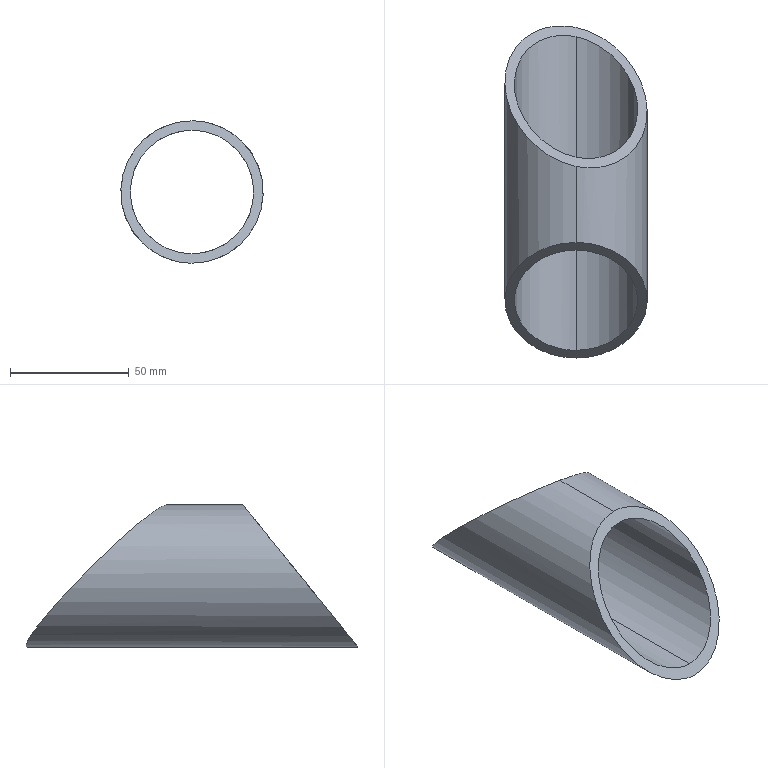Part | SolidWorks | features BaseBody 1 | 1 solid | 6 faces | box 60 x 140 x 60 mm | volume 60313 mm3 | cylinder 4 | plane 2 | commonest cylinder face diameters 52 x2 60 x2
STEP:
#1=CARTESIAN_POINT('',(0.,84.568,26.));
#2=VERTEX_POINT('',#1);
#3=CARTESIAN_POINT('',(0.,135.432,-26.));
#4=VERTEX_POINT('',#3);
#5=CARTESIAN_POINT('',(0.,84.568,26.));
#6=CARTESIAN_POINT('',(-52.,95.38,26.));
#7=CARTESIAN_POINT('',(-52.,146.243,-26.));
#8=CARTESIAN_POINT('',(0.,135.432,-26.));
#9=(BOUNDED_CURVE()B_SPLINE_CURVE(3,(#5,#6,#7,#8),.UNSPECIFIED.,.F.,.T.)B_SPLINE_CURVE_WITH_KNOTS((4,4),(0.2094,3.351),.UNSPECIFIED.)CURVE()GEOMETRIC_REPRESENTATION_ITEM()RATIONAL_B_SPLINE_CURVE((1.,0.3333,0.3333,1.))REPRESENTATION_ITEM(''));
#10=EDGE_CURVE('',#2,#4,#9,.T.);
#11=ORIENTED_EDGE('',*,*,#10,.F.);
#12=CARTESIAN_POINT('',(0.,45.348,26.));
#13=VERTEX_POINT('',#12);
#14=CARTESIAN_POINT('',(0.,140.,26.));
#15=DIRECTION('',(0.,-1.,0.));
#16=VECTOR('',#15,1000.);
#17=LINE('',#14,#16);
#18=EDGE_CURVE('',#2,#13,#17,.T.);
#19=ORIENTED_EDGE('',*,*,#18,.T.);
#20=CARTESIAN_POINT('',(0.,3.239,-26.));
#21=VERTEX_POINT('',#20);
#22=CARTESIAN_POINT('',(0.,45.348,26.));
#23=CARTESIAN_POINT('',(-52.,45.348,26.));
#24=CARTESIAN_POINT('',(-52.,3.239,-26.));
#25=CARTESIAN_POINT('',(0.,3.239,-26.));
#26=(BOUNDED_CURVE()B_SPLINE_CURVE(3,(#22,#23,#24,#25),.UNSPECIFIED.,.F.,.T.)B_SPLINE_CURVE_WITH_KNOTS((4,4),(3.142,6.283),.UNSPECIFIED.)CURVE()GEOMETRIC_REPRESENTATION_ITEM()RATIONAL_B_SPLINE_CURVE((1.,0.3333,0.3333,1.))REPRESENTATION_ITEM(''));
#27=EDGE_CURVE('',#13,#21,#26,.T.);
#28=ORIENTED_EDGE('',*,*,#27,.T.);
#29=CARTESIAN_POINT('',(0.,140.,-26.));
#30=DIRECTION('',(0.,-1.,0.));
#31=VECTOR('',#30,1000.);
#32=LINE('',#29,#31);
#33=EDGE_CURVE('',#4,#21,#32,.T.);
#34=ORIENTED_EDGE('',*,*,#33,.F.);
#35=EDGE_LOOP('',(#11,#19,#28,#34));
#36=FACE_OUTER_BOUND('',#35,.T.);
#37=CARTESIAN_POINT('',(0.,140.,0.));
#38=DIRECTION('',(0.,-1.,0.));
#39=DIRECTION('',(0.,0.,-1.));
#40=AXIS2_PLACEMENT_3D('',#37,#38,#39);
#41=CYLINDRICAL_SURFACE('',#40,26.);
#42=ADVANCED_FACE('',(#36),#41,.F.);
#43=CARTESIAN_POINT('',(0.,139.344,-30.));
#44=VERTEX_POINT('',#43);
#45=CARTESIAN_POINT('',(0.,80.656,30.));
#46=VERTEX_POINT('',#45);
#47=CARTESIAN_POINT('',(0.,139.344,-30.));
#48=CARTESIAN_POINT('',(60.,126.87,-30.));
#49=CARTESIAN_POINT('',(60.,68.181,30.));
#50=CARTESIAN_POINT('',(0.,80.656,30.));
#51=(BOUNDED_CURVE()B_SPLINE_CURVE(3,(#47,#48,#49,#50),.UNSPECIFIED.,.F.,.F.)B_SPLINE_CURVE_WITH_KNOTS((4,4),(3.351,6.493),.UNSPECIFIED.)CURVE()GEOMETRIC_REPRESENTATION_ITEM()RATIONAL_B_SPLINE_CURVE((1.,0.3333,0.3333,1.))REPRESENTATION_ITEM(''));
#52=EDGE_CURVE('',#44,#46,#51,.T.);
#53=ORIENTED_EDGE('',*,*,#52,.T.);
#54=CARTESIAN_POINT('',(0.,48.587,30.));
#55=VERTEX_POINT('',#54);
#56=CARTESIAN_POINT('',(0.,140.,30.));
#57=DIRECTION('',(0.,-1.,0.));
#58=VECTOR('',#57,1000.);
#59=LINE('',#56,#58);
#60=EDGE_CURVE('',#46,#55,#59,.T.);
#61=ORIENTED_EDGE('',*,*,#60,.T.);
#62=CARTESIAN_POINT('',(0.,0.,-30.));
#63=VERTEX_POINT('',#62);
#64=CARTESIAN_POINT('',(0.,0.,-30.));
#65=CARTESIAN_POINT('',(60.,0.,-30.));
#66=CARTESIAN_POINT('',(60.,48.587,30.));
#67=CARTESIAN_POINT('',(0.,48.587,30.));
#68=(BOUNDED_CURVE()B_SPLINE_CURVE(3,(#64,#65,#66,#67),.UNSPECIFIED.,.F.,.T.)B_SPLINE_CURVE_WITH_KNOTS((4,4),(0.,3.142),.UNSPECIFIED.)CURVE()GEOMETRIC_REPRESENTATION_ITEM()RATIONAL_B_SPLINE_CURVE((1.,0.3333,0.3333,1.))REPRESENTATION_ITEM(''));
#69=EDGE_CURVE('',#63,#55,#68,.T.);
#70=ORIENTED_EDGE('',*,*,#69,.F.);
#71=CARTESIAN_POINT('',(0.,140.,-30.));
#72=DIRECTION('',(0.,-1.,0.));
#73=VECTOR('',#72,1000.);
#74=LINE('',#71,#73);
#75=EDGE_CURVE('',#44,#63,#74,.T.);
#76=ORIENTED_EDGE('',*,*,#75,.F.);
#77=EDGE_LOOP('',(#53,#61,#70,#76));
#78=FACE_OUTER_BOUND('',#77,.T.);
#79=CARTESIAN_POINT('',(0.,140.,0.));
#80=DIRECTION('',(0.,-1.,0.));
#81=DIRECTION('',(0.,0.,-1.));
#82=AXIS2_PLACEMENT_3D('',#79,#80,#81);
#83=CYLINDRICAL_SURFACE('',#82,30.);
#84=ADVANCED_FACE('',(#78),#83,.T.);
#85=ORIENTED_EDGE('',*,*,#60,.F.);
#86=CARTESIAN_POINT('',(0.,80.656,30.));
#87=CARTESIAN_POINT('',(-60.,93.13,30.));
#88=CARTESIAN_POINT('',(-60.,151.819,-30.));
#89=CARTESIAN_POINT('',(0.,139.344,-30.));
#90=(BOUNDED_CURVE()B_SPLINE_CURVE(3,(#86,#87,#88,#89),.UNSPECIFIED.,.F.,.F.)B_SPLINE_CURVE_WITH_KNOTS((4,4),(0.2094,3.351),.UNSPECIFIED.)CURVE()GEOMETRIC_REPRESENTATION_ITEM()RATIONAL_B_SPLINE_CURVE((1.,0.3333,0.3333,1.))REPRESENTATION_ITEM(''));
#91=EDGE_CURVE('',#46,#44,#90,.T.);
#92=ORIENTED_EDGE('',*,*,#91,.T.);
#93=ORIENTED_EDGE('',*,*,#75,.T.);
#94=CARTESIAN_POINT('',(0.,48.587,30.));
#95=CARTESIAN_POINT('',(-60.,48.587,30.));
#96=CARTESIAN_POINT('',(-60.,0.,-30.));
#97=CARTESIAN_POINT('',(0.,0.,-30.));
#98=(BOUNDED_CURVE()B_SPLINE_CURVE(3,(#94,#95,#96,#97),.UNSPECIFIED.,.F.,.F.)B_SPLINE_CURVE_WITH_KNOTS((4,4),(3.142,6.283),.UNSPECIFIED.)CURVE()GEOMETRIC_REPRESENTATION_ITEM()RATIONAL_B_SPLINE_CURVE((1.,0.3333,0.3333,1.))REPRESENTATION_ITEM(''));
#99=EDGE_CURVE('',#55,#63,#98,.T.);
#100=ORIENTED_EDGE('',*,*,#99,.F.);
#101=EDGE_LOOP('',(#85,#92,#93,#100));
#102=FACE_OUTER_BOUND('',#101,.T.);
#103=CARTESIAN_POINT('',(0.,140.,0.));
#104=DIRECTION('',(0.,-1.,0.));
#105=DIRECTION('',(0.,0.,-1.));
#106=AXIS2_PLACEMENT_3D('',#103,#104,#105);
#107=CYLINDRICAL_SURFACE('',#106,30.);
#108=ADVANCED_FACE('',(#102),#107,.T.);
#109=ORIENTED_EDGE('',*,*,#18,.F.);
#110=CARTESIAN_POINT('',(0.,135.432,-26.));
#111=CARTESIAN_POINT('',(52.,124.62,-26.));
#112=CARTESIAN_POINT('',(52.,73.757,26.));
#113=CARTESIAN_POINT('',(0.,84.568,26.));
#114=(BOUNDED_CURVE()B_SPLINE_CURVE(3,(#110,#111,#112,#113),.UNSPECIFIED.,.F.,.F.)B_SPLINE_CURVE_WITH_KNOTS((4,4),(3.351,6.493),.UNSPECIFIED.)CURVE()GEOMETRIC_REPRESENTATION_ITEM()RATIONAL_B_SPLINE_CURVE((1.,0.3333,0.3333,1.))REPRESENTATION_ITEM(''));
#115=EDGE_CURVE('',#4,#2,#114,.T.);
#116=ORIENTED_EDGE('',*,*,#115,.F.);
#117=ORIENTED_EDGE('',*,*,#33,.T.);
#118=CARTESIAN_POINT('',(0.,3.239,-26.));
#119=CARTESIAN_POINT('',(52.,3.239,-26.));
#120=CARTESIAN_POINT('',(52.,45.348,26.));
#121=CARTESIAN_POINT('',(0.,45.348,26.));
#122=(BOUNDED_CURVE()B_SPLINE_CURVE(3,(#118,#119,#120,#121),.UNSPECIFIED.,.F.,.F.)B_SPLINE_CURVE_WITH_KNOTS((4,4),(0.,3.142),.UNSPECIFIED.)CURVE()GEOMETRIC_REPRESENTATION_ITEM()RATIONAL_B_SPLINE_CURVE((1.,0.3333,0.3333,1.))REPRESENTATION_ITEM(''));
#123=EDGE_CURVE('',#21,#13,#122,.T.);
#124=ORIENTED_EDGE('',*,*,#123,.T.);
#125=EDGE_LOOP('',(#109,#116,#117,#124));
#126=FACE_OUTER_BOUND('',#125,.T.);
#127=CARTESIAN_POINT('',(0.,140.,0.));
#128=DIRECTION('',(0.,-1.,0.));
#129=DIRECTION('',(0.,0.,-1.));
#130=AXIS2_PLACEMENT_3D('',#127,#128,#129);
#131=CYLINDRICAL_SURFACE('',#130,26.);
#132=ADVANCED_FACE('',(#126),#131,.F.);
#133=ORIENTED_EDGE('',*,*,#69,.T.);
#134=ORIENTED_EDGE('',*,*,#99,.T.);
#135=EDGE_LOOP('',(#133,#134));
#136=FACE_OUTER_BOUND('',#135,.T.);
#137=ORIENTED_EDGE('',*,*,#123,.F.);
#138=ORIENTED_EDGE('',*,*,#27,.F.);
#139=EDGE_LOOP('',(#137,#138));
#140=FACE_BOUND('',#139,.T.);
#141=CARTESIAN_POINT('',(204.634,0.,-30.));
#142=DIRECTION('',(0.,-0.7771,0.6293));
#143=DIRECTION('',(-1.,0.,0.));
#144=AXIS2_PLACEMENT_3D('',#141,#142,#143);
#145=PLANE('',#144);
#146=ADVANCED_FACE('',(#136,#140),#145,.T.);
#147=ORIENTED_EDGE('',*,*,#52,.F.);
#148=ORIENTED_EDGE('',*,*,#91,.F.);
#149=EDGE_LOOP('',(#147,#148));
#150=FACE_OUTER_BOUND('',#149,.T.);
#151=ORIENTED_EDGE('',*,*,#115,.T.);
#152=ORIENTED_EDGE('',*,*,#10,.T.);
#153=EDGE_LOOP('',(#151,#152));
#154=FACE_BOUND('',#153,.T.);
#155=CARTESIAN_POINT('',(201.551,140.,-73.511));
#156=DIRECTION('',(-0.147,-0.7071,-0.6917));
#157=DIRECTION('',(0.,0.6993,-0.7149));
#158=AXIS2_PLACEMENT_3D('',#155,#156,#157);
#159=PLANE('',#158);
#160=ADVANCED_FACE('',(#150,#154),#159,.F.);
#161=CLOSED_SHELL('',(#42,#84,#108,#132,#146,#160));
#162=MANIFOLD_SOLID_BREP('',#161);
#163=CARTESIAN_POINT('',(0.,0.,0.));
#164=DIRECTION('',(0.,0.,1.));
#165=DIRECTION('',(1.,0.,0.));
#166=AXIS2_PLACEMENT_3D('',#163,#164,#165);
#167=(LENGTH_UNIT()NAMED_UNIT(*)SI_UNIT(.MILLI.,.METRE.));
#168=UNCERTAINTY_MEASURE_WITH_UNIT(LENGTH_MEASURE(0.00001),#167,'','');
#169=(NAMED_UNIT(*)PLANE_ANGLE_UNIT()SI_UNIT($,.RADIAN.));
#170=(NAMED_UNIT(*)SI_UNIT($,.STERADIAN.)SOLID_ANGLE_UNIT());
#171=(GEOMETRIC_REPRESENTATION_CONTEXT(3)GLOBAL_UNCERTAINTY_ASSIGNED_CONTEXT((#168))GLOBAL_UNIT_ASSIGNED_CONTEXT((#167,#169,#170))REPRESENTATION_CONTEXT('',''));
#172=ADVANCED_BREP_SHAPE_REPRESENTATION('',(#162,#166),#171);